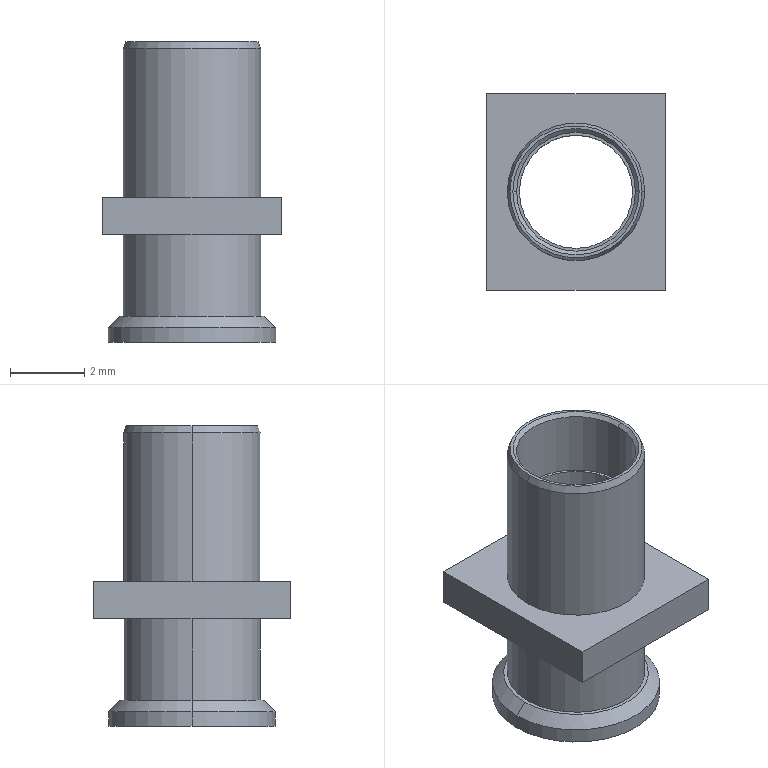Part | STEP file | Rivet_Default | 1 solid | 31 faces | box 4.8 x 5.3 x 8.1 mm | volume 41.537 mm3 | cylinder 12 | plane 11 | cone 8 | commonest cylinder face diameters 3.2 x4 3.7 x4 3.048 x2 4.5 x2